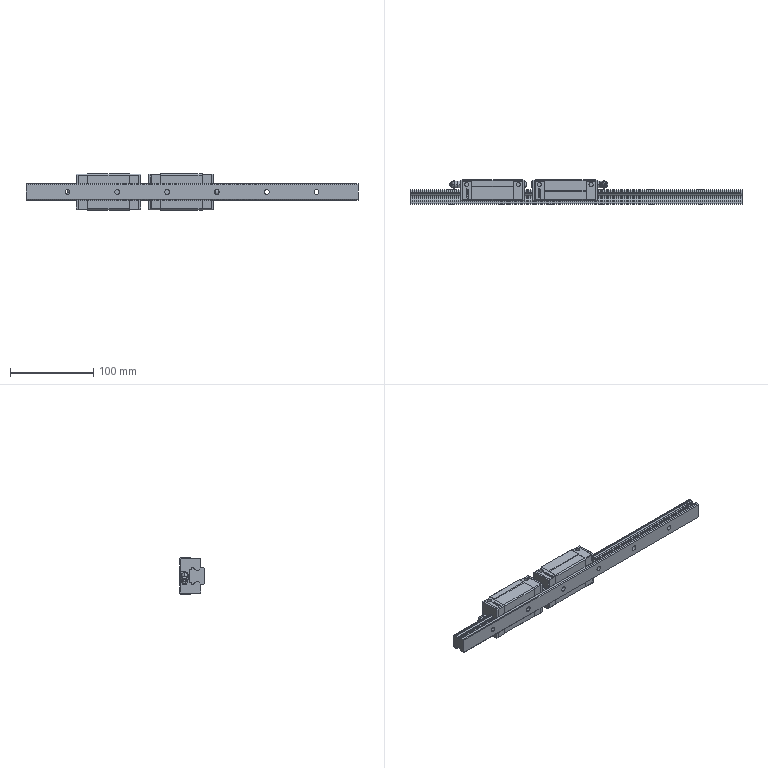Part | SolidWorks | 15 solids | 1711 faces | box 400 x 30 x 44 mm | volume 248543 mm3 | plane 1058 | cylinder 474 | cone 92 | spline 69 | sphere 12 | torus 6 | commonest cylinder face diameters 1 x148 0.2 x68 2 x58 4.06 x44 0.1 x36 6 x36